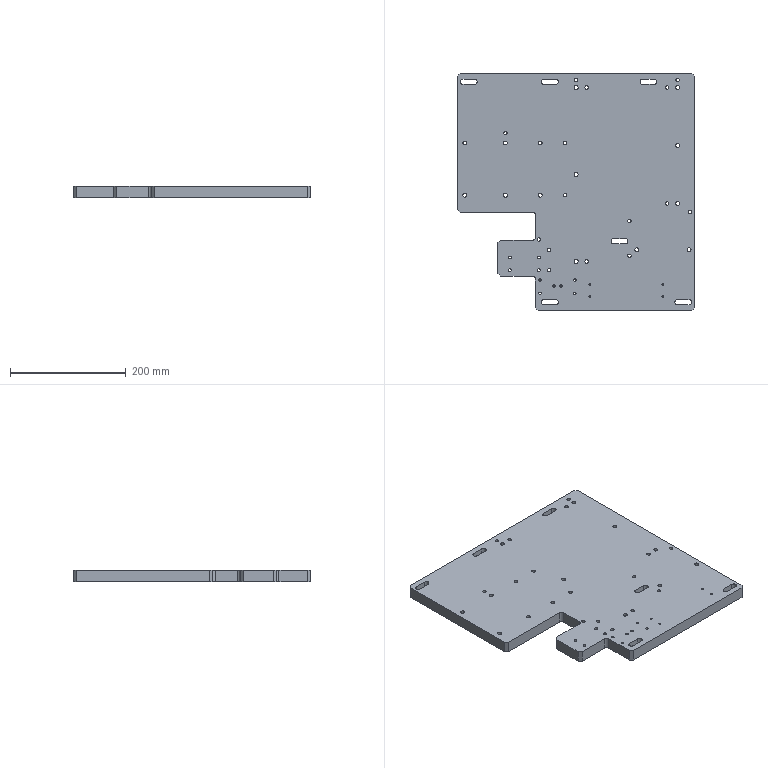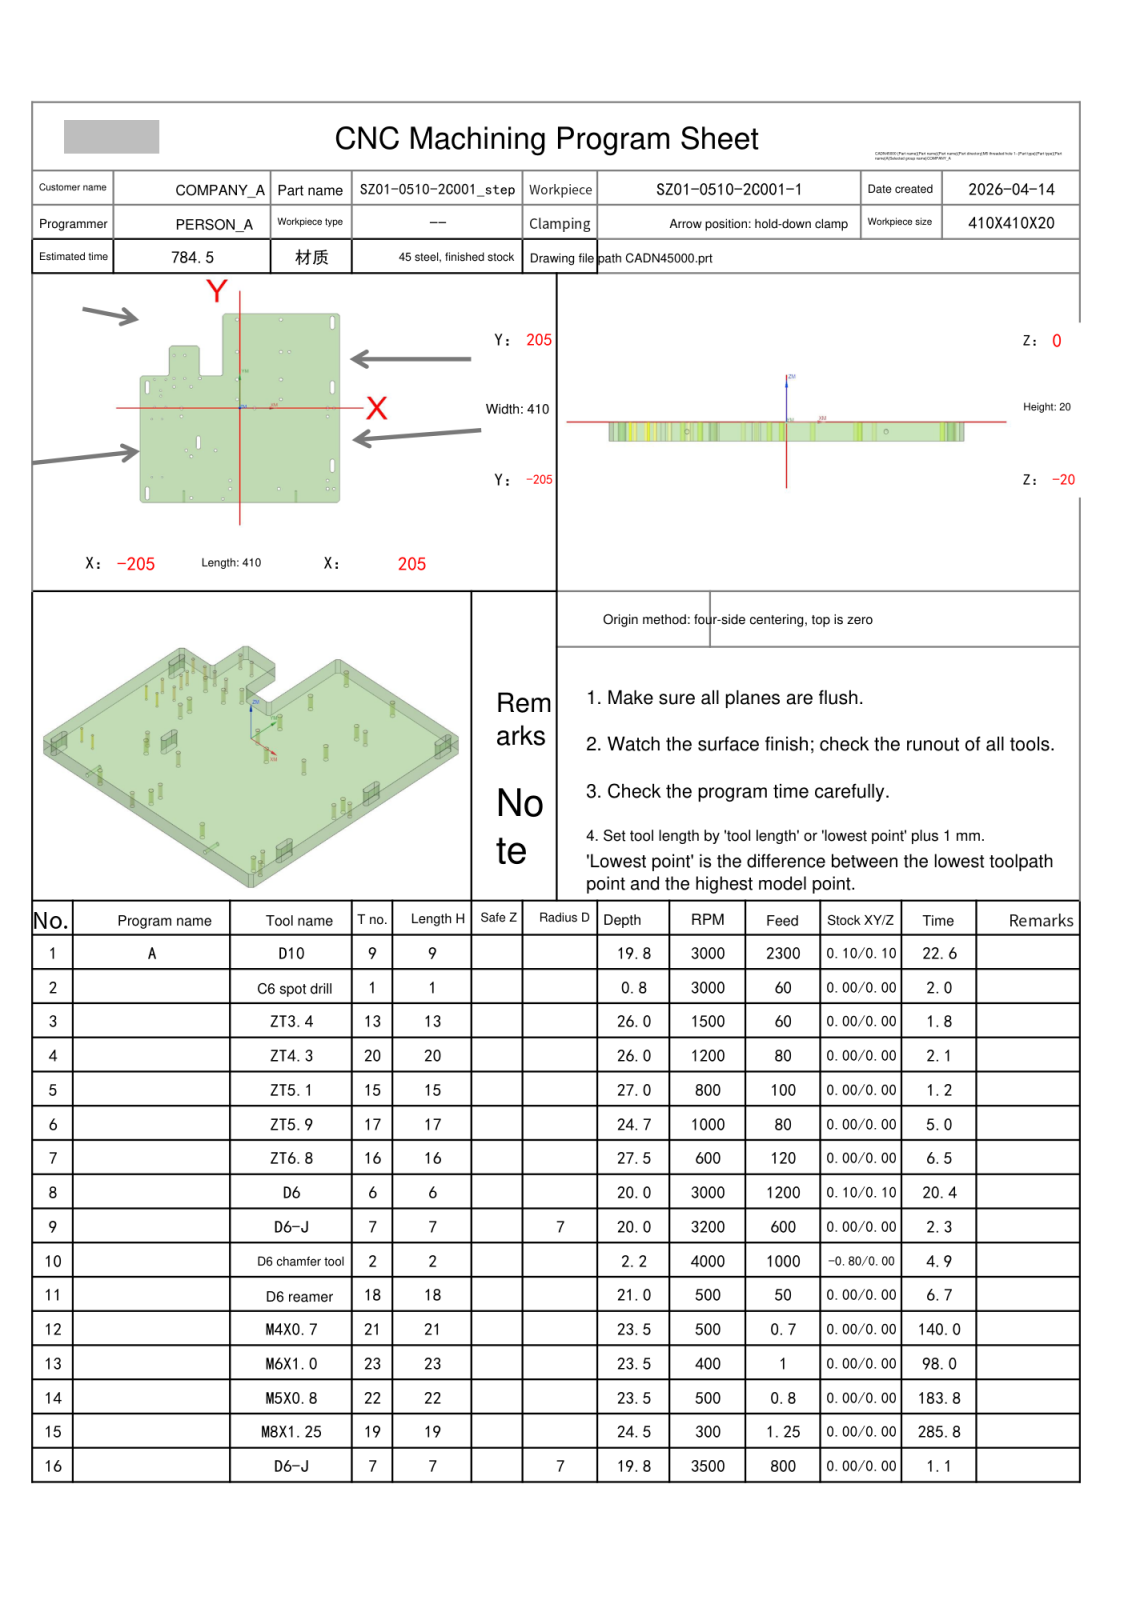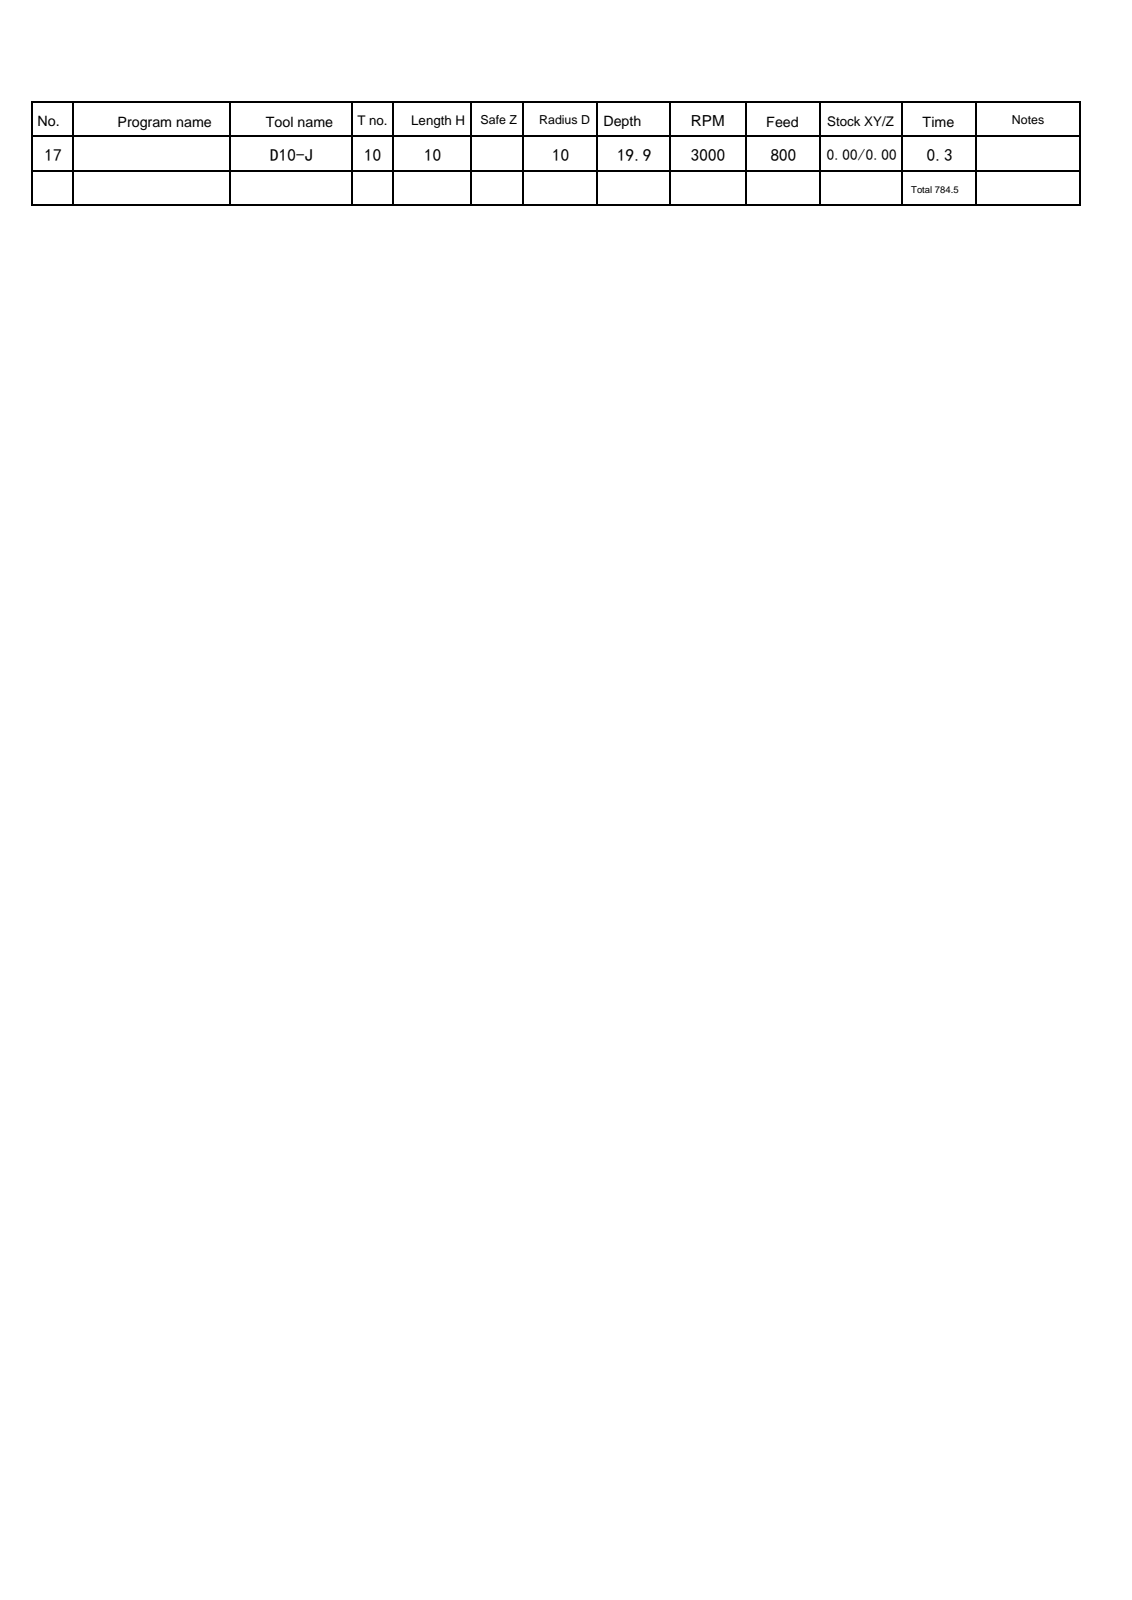NC program | NX | posted by the shop | part box 410 x 410 x 20 mm
Lines 3112 to 3293 of 7905:
N2 T01 M06
(C6 spot drill  D=6. R=0. H=01 ce=0.00 di=0.10)
G00 G90 G54 X-5.5 Y121.85 M03 S3000
G43 H01 Z50.
M08
G98 G81 X-5.5 Y121.85 Z-.8 R1. F60.
Y191.85
X84.5
X101.47 Y121.85
X84.5
Y61.85
Y18.85
X30.2 Y-.2
X-5.5 Y18.85
Y61.85
X-82. Y64.215
X-100. Y46.215
X-113. Y64.215
Y114.215
X-135.
Y64.215
Y46.215
X-152. Y62.
X-175.
X-162.5 Y37.96
Y25.96
X-175. Y2.
X-180.5 Y-24.
X-159.5
X-152. Y2.
X-119.8 Y-.2
Y-18.2
X-50. Y-92.
X-99.745 Y-105.
X-110. Y-92.
X-180.5 Y-150.
X-159.5
X-99.745 Y-195.
X-34.7 Y-197.
X-19.8 Y-175.2
Y-157.2
X80.2 Y-175.2
X180.2
X193.2
X180.2 Y-157.2
Y-18.2
Y-.2
X193.2
X-190. Y55.
Y35.
Y-175.
Y-195.
X-85. Y-65.
Y-85.
X190. Y-115.
Y-135.
Y55.
Y35.
Y195.
Y175.
G80
G00 Z50.
G91 G28 Z0.0
M05
M09
G91 G28 Z0.0
M01
N3 T13 M06
(ZT3.4 D=3.4 DR_a=118 H=13)
G00 G90 G54 X-159.5 Y-24. M03 S1500
G43 H13 Z50.
M08
G98 G83 X-159.5 Y-24. Z-26. R1. F60. Q1.
X-180.5
Y-150.
X-159.5
G80
G00 Z50.
G91 G28 Z0.0
M05
M09
G91 G28 Z0.0
M01
N4 T20 M06
(ZT4.3 D=4.3 DR_a=118 H=20)
G00 G90 G54 X-175. Y2. M03 S1200
G43 H20 Z50.
M08
G98 G83 X-175. Y2. Z-26. R1. F80. Q1.5
X-152.
X-162.5 Y25.96
Y37.96
X-152. Y62.
X-175.
G80
G00 Z50.
G91 G28 Z0.0
M05
M09
G91 G28 Z0.0
M01
N5 T15 M06
(ZT5.1 D=5.1 DR_a=118 H=15)
G00 G90 G54 X-135. Y64.215 M03 S800
G43 H15 Z50.
M08
G98 G83 X-135. Y64.215 Z-27. R1. F100. Q2.
X-113.
Y114.215
X-135.
G80
G00 Z50.
G91 G28 Z0.0
M05
M09
G91 G28 Z0.0
M01
N6 T17 M06
(ZT5.9 D=5.9 DR_a=120 H=17)
G00 G90 G54 X-34.7 Y-197. M03 S1000
G43 H17 Z50.
M08
G98 G83 X-34.7 Y-197. Z-24.703 R1. F80. Q1.
X-19.8 Y-157.2
X-50. Y-92.
X-110.
X-119.8 Y-18.2
X-135. Y46.215
X-100.
X-82. Y64.215
X-5.5 Y18.85
X84.5
X101.47 Y121.85
X193.2 Y-.2
X180.2 Y-18.2
Y-157.2
X193.2 Y-175.2
G80
G00 Z50.
G91 G28 Z0.0
M05
M09
G91 G28 Z0.0
M01
N7 T16 M06
(ZT6.8 D=6.8 DR_a=118 H=16)
G00 G90 G54 X180.2 Y-175.2 M03 S600
G43 H16 Z50.
M08
G98 G83 X180.2 Y-175.2 Z-27.543 R1. F120. Q2.
X80.2
X-19.8
X-99.745 Y-195.
Y-105.
X-119.8 Y-.2
X30.2
X-5.5 Y61.85
Y121.85
Y191.85
X84.5
Y121.85
Y61.85
X180.2 Y-.2
X-190. Y55.
Y35.
Y-175.
Y-195.
X-85. Y-65.
Y-85.
X190. Y-115.
Y-135.
Y55.
Y35.
Y195.
Y175.
G80
G00 Z50.
G91 G28 Z0.0
M05
M09
G91 G28 Z0.0
M01